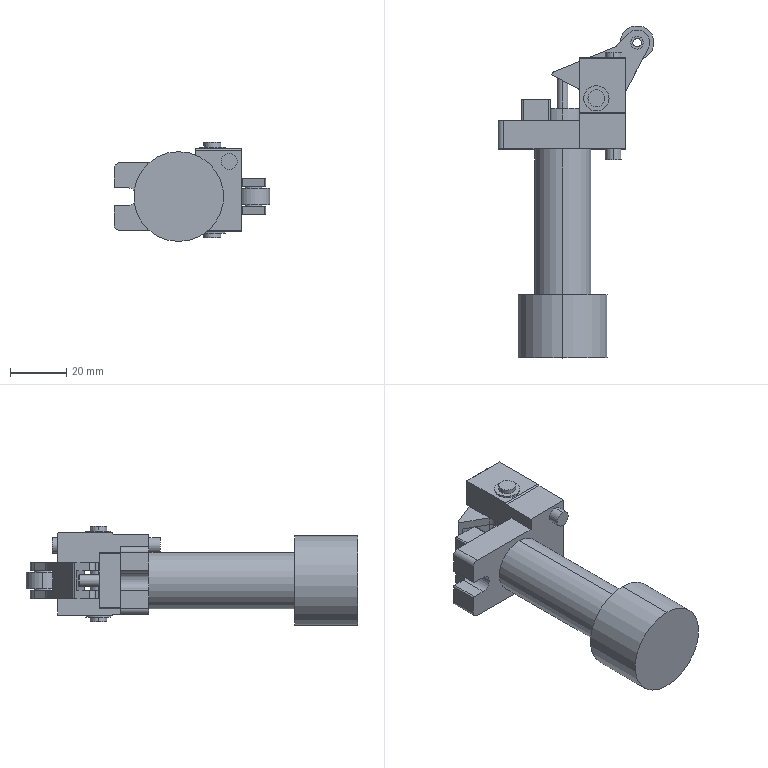Part | STEP file | TWH-S-32x20-K F-1-P_r-0 | 1 solid | 137 faces | box 55.5 x 118.212 x 35.25 mm | volume 58863 mm3 | cylinder 69 | plane 62 | cone 4 | torus 2 | commonest cylinder face diameters 6 x14 1 x9 4 x8 9 x6 2 x4 4.5 x4